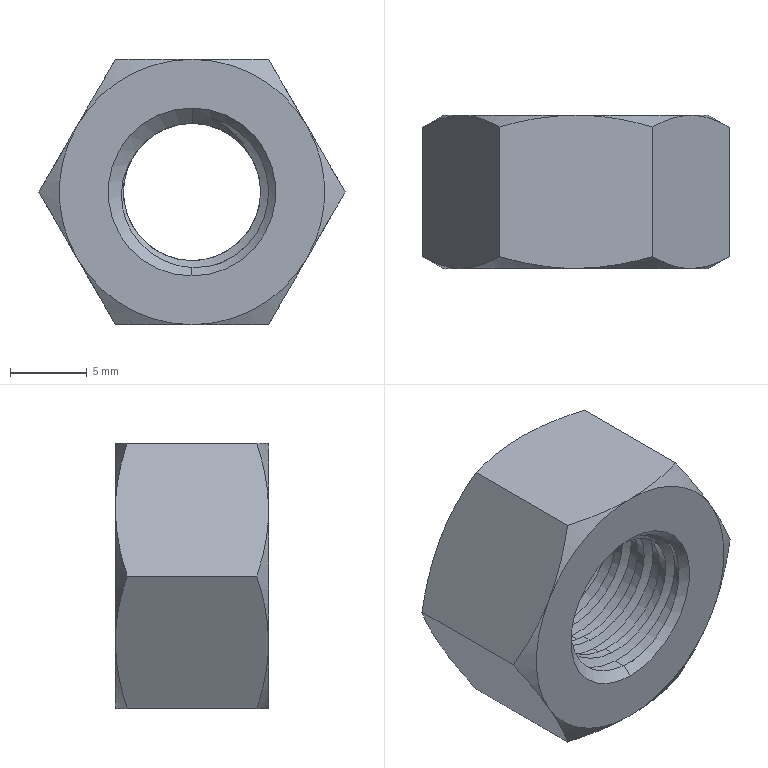Part | SolidWorks | features ICE 2, Chamfer 1, CombineBodies 1, Extrusion 1, MoveCopyBody 1, Stock 1 | 1 solid | 46 faces | box 20 x 10 x 17.321 mm | volume 1854 mm3 | cylinder 20 | cone 16 | plane 8 | spline 2 | commonest cylinder face diameters 8.96 x10 10 x10